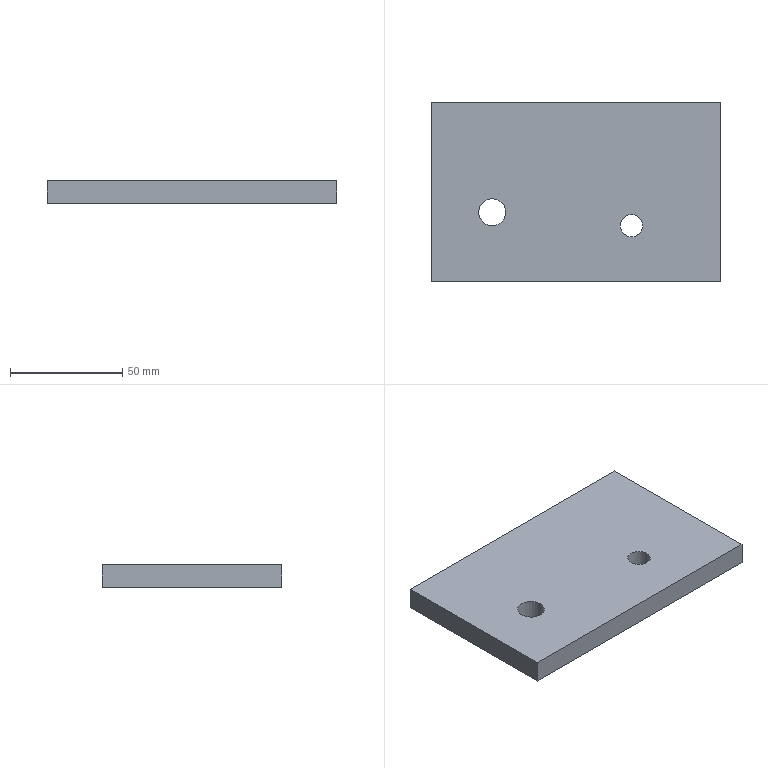Part | NX | features solid 2 | 1 solid | 8 faces | box 129 x 80 x 10 mm | volume 101284 mm3 | plane 6 | cylinder 2 | commonest cylinder face diameters 10 x1 12 x1
STEP:
#1=CARTESIAN_POINT('',(-391.,441.,-10.));
#2=VERTEX_POINT('',#1);
#3=CARTESIAN_POINT('',(-397.,441.,-10.));
#4=DIRECTION('',(0.,0.,1.));
#5=DIRECTION('',(1.,0.,0.));
#6=AXIS2_PLACEMENT_3D('',#3,#4,#5);
#7=CIRCLE('',#6,6.);
#8=EDGE_CURVE('',#2,#2,#7,.F.);
#9=ORIENTED_EDGE('',*,*,#8,.T.);
#10=EDGE_LOOP('',(#9));
#11=FACE_BOUND('',#10,.T.);
#12=CARTESIAN_POINT('',(-424.173,490.,-10.));
#13=VERTEX_POINT('',#12);
#14=CARTESIAN_POINT('',(-295.173,490.,-10.));
#15=VERTEX_POINT('',#14);
#16=CARTESIAN_POINT('',(-374.173,490.,-10.));
#17=DIRECTION('',(1.,0.,0.));
#18=VECTOR('',#17,1000.);
#19=LINE('',#16,#18);
#20=EDGE_CURVE('',#13,#15,#19,.T.);
#21=ORIENTED_EDGE('',*,*,#20,.F.);
#22=CARTESIAN_POINT('',(-424.173,410.,-10.));
#23=VERTEX_POINT('',#22);
#24=CARTESIAN_POINT('',(-424.173,460.,-10.));
#25=DIRECTION('',(0.,-1.,0.));
#26=VECTOR('',#25,1000.);
#27=LINE('',#24,#26);
#28=EDGE_CURVE('',#13,#23,#27,.T.);
#29=ORIENTED_EDGE('',*,*,#28,.T.);
#30=CARTESIAN_POINT('',(-295.173,410.,-10.));
#31=VERTEX_POINT('',#30);
#32=CARTESIAN_POINT('',(-374.173,410.,-10.));
#33=DIRECTION('',(-1.,0.,0.));
#34=VECTOR('',#33,1000.);
#35=LINE('',#32,#34);
#36=EDGE_CURVE('',#31,#23,#35,.T.);
#37=ORIENTED_EDGE('',*,*,#36,.F.);
#38=CARTESIAN_POINT('',(-295.173,410.,-10.));
#39=DIRECTION('',(0.,1.,0.));
#40=VECTOR('',#39,1000.);
#41=LINE('',#38,#40);
#42=EDGE_CURVE('',#31,#15,#41,.T.);
#43=ORIENTED_EDGE('',*,*,#42,.T.);
#44=EDGE_LOOP('',(#21,#29,#37,#43));
#45=FACE_BOUND('',#44,.T.);
#46=CARTESIAN_POINT('',(-330.,435.,-10.));
#47=VERTEX_POINT('',#46);
#48=CARTESIAN_POINT('',(-335.,435.,-10.));
#49=DIRECTION('',(0.,0.,1.));
#50=DIRECTION('',(1.,0.,0.));
#51=AXIS2_PLACEMENT_3D('',#48,#49,#50);
#52=CIRCLE('',#51,5.);
#53=EDGE_CURVE('',#47,#47,#52,.F.);
#54=ORIENTED_EDGE('',*,*,#53,.T.);
#55=EDGE_LOOP('',(#54));
#56=FACE_BOUND('',#55,.T.);
#57=CARTESIAN_POINT('',(-374.173,460.,-10.));
#58=DIRECTION('',(0.,0.,1.));
#59=DIRECTION('',(1.,0.,0.));
#60=AXIS2_PLACEMENT_3D('',#57,#58,#59);
#61=PLANE('',#60);
#62=ADVANCED_FACE('',(#11,#45,#56),#61,.T.);
#63=CARTESIAN_POINT('',(-424.173,490.,-20.));
#64=VERTEX_POINT('',#63);
#65=CARTESIAN_POINT('',(-424.173,410.,-20.));
#66=VERTEX_POINT('',#65);
#67=CARTESIAN_POINT('',(-424.173,460.,-20.));
#68=DIRECTION('',(0.,-1.,0.));
#69=VECTOR('',#68,1000.);
#70=LINE('',#67,#69);
#71=EDGE_CURVE('',#64,#66,#70,.T.);
#72=ORIENTED_EDGE('',*,*,#71,.F.);
#73=CARTESIAN_POINT('',(-295.173,490.,-20.));
#74=VERTEX_POINT('',#73);
#75=CARTESIAN_POINT('',(-374.173,490.,-20.));
#76=DIRECTION('',(1.,0.,0.));
#77=VECTOR('',#76,1000.);
#78=LINE('',#75,#77);
#79=EDGE_CURVE('',#64,#74,#78,.T.);
#80=ORIENTED_EDGE('',*,*,#79,.T.);
#81=CARTESIAN_POINT('',(-295.173,410.,-20.));
#82=VERTEX_POINT('',#81);
#83=CARTESIAN_POINT('',(-295.173,410.,-20.));
#84=DIRECTION('',(0.,1.,0.));
#85=VECTOR('',#84,1000.);
#86=LINE('',#83,#85);
#87=EDGE_CURVE('',#82,#74,#86,.T.);
#88=ORIENTED_EDGE('',*,*,#87,.F.);
#89=CARTESIAN_POINT('',(-374.173,410.,-20.));
#90=DIRECTION('',(-1.,0.,0.));
#91=VECTOR('',#90,1000.);
#92=LINE('',#89,#91);
#93=EDGE_CURVE('',#82,#66,#92,.T.);
#94=ORIENTED_EDGE('',*,*,#93,.T.);
#95=EDGE_LOOP('',(#72,#80,#88,#94));
#96=FACE_BOUND('',#95,.T.);
#97=CARTESIAN_POINT('',(-391.,441.,-20.));
#98=VERTEX_POINT('',#97);
#99=CARTESIAN_POINT('',(-397.,441.,-20.));
#100=DIRECTION('',(0.,0.,1.));
#101=DIRECTION('',(1.,0.,0.));
#102=AXIS2_PLACEMENT_3D('',#99,#100,#101);
#103=CIRCLE('',#102,6.);
#104=EDGE_CURVE('',#98,#98,#103,.F.);
#105=ORIENTED_EDGE('',*,*,#104,.F.);
#106=EDGE_LOOP('',(#105));
#107=FACE_BOUND('',#106,.T.);
#108=CARTESIAN_POINT('',(-330.,435.,-20.));
#109=VERTEX_POINT('',#108);
#110=CARTESIAN_POINT('',(-335.,435.,-20.));
#111=DIRECTION('',(0.,0.,-1.));
#112=DIRECTION('',(1.,0.,0.));
#113=AXIS2_PLACEMENT_3D('',#110,#111,#112);
#114=CIRCLE('',#113,5.);
#115=EDGE_CURVE('',#109,#109,#114,.T.);
#116=ORIENTED_EDGE('',*,*,#115,.F.);
#117=EDGE_LOOP('',(#116));
#118=FACE_BOUND('',#117,.T.);
#119=CARTESIAN_POINT('',(-374.173,460.,-20.));
#120=DIRECTION('',(0.,0.,1.));
#121=DIRECTION('',(1.,0.,0.));
#122=AXIS2_PLACEMENT_3D('',#119,#120,#121);
#123=PLANE('',#122);
#124=ADVANCED_FACE('',(#96,#107,#118),#123,.F.);
#125=ORIENTED_EDGE('',*,*,#87,.T.);
#126=CARTESIAN_POINT('',(-295.173,490.,-10.));
#127=DIRECTION('',(0.,0.,-1.));
#128=VECTOR('',#127,1000.);
#129=LINE('',#126,#128);
#130=EDGE_CURVE('',#15,#74,#129,.T.);
#131=ORIENTED_EDGE('',*,*,#130,.F.);
#132=ORIENTED_EDGE('',*,*,#42,.F.);
#133=CARTESIAN_POINT('',(-295.173,410.,-10.));
#134=DIRECTION('',(0.,0.,-1.));
#135=VECTOR('',#134,1000.);
#136=LINE('',#133,#135);
#137=EDGE_CURVE('',#31,#82,#136,.T.);
#138=ORIENTED_EDGE('',*,*,#137,.T.);
#139=EDGE_LOOP('',(#125,#131,#132,#138));
#140=FACE_BOUND('',#139,.T.);
#141=CARTESIAN_POINT('',(-295.173,410.,-10.));
#142=DIRECTION('',(-1.,0.,0.));
#143=DIRECTION('',(0.,-1.,0.));
#144=AXIS2_PLACEMENT_3D('',#141,#142,#143);
#145=PLANE('',#144);
#146=ADVANCED_FACE('',(#140),#145,.F.);
#147=ORIENTED_EDGE('',*,*,#71,.T.);
#148=CARTESIAN_POINT('',(-424.173,410.,-10.));
#149=DIRECTION('',(0.,0.,-1.));
#150=VECTOR('',#149,1000.);
#151=LINE('',#148,#150);
#152=EDGE_CURVE('',#23,#66,#151,.T.);
#153=ORIENTED_EDGE('',*,*,#152,.F.);
#154=ORIENTED_EDGE('',*,*,#28,.F.);
#155=CARTESIAN_POINT('',(-424.173,490.,-10.));
#156=DIRECTION('',(0.,0.,-1.));
#157=VECTOR('',#156,1000.);
#158=LINE('',#155,#157);
#159=EDGE_CURVE('',#13,#64,#158,.T.);
#160=ORIENTED_EDGE('',*,*,#159,.T.);
#161=EDGE_LOOP('',(#147,#153,#154,#160));
#162=FACE_BOUND('',#161,.T.);
#163=CARTESIAN_POINT('',(-424.173,460.,-10.));
#164=DIRECTION('',(1.,0.,0.));
#165=DIRECTION('',(0.,1.,0.));
#166=AXIS2_PLACEMENT_3D('',#163,#164,#165);
#167=PLANE('',#166);
#168=ADVANCED_FACE('',(#162),#167,.F.);
#169=ORIENTED_EDGE('',*,*,#137,.F.);
#170=ORIENTED_EDGE('',*,*,#36,.T.);
#171=ORIENTED_EDGE('',*,*,#152,.T.);
#172=ORIENTED_EDGE('',*,*,#93,.F.);
#173=EDGE_LOOP('',(#169,#170,#171,#172));
#174=FACE_BOUND('',#173,.T.);
#175=CARTESIAN_POINT('',(-374.173,410.,-10.));
#176=DIRECTION('',(0.,1.,0.));
#177=DIRECTION('',(-1.,0.,0.));
#178=AXIS2_PLACEMENT_3D('',#175,#176,#177);
#179=PLANE('',#178);
#180=ADVANCED_FACE('',(#174),#179,.F.);
#181=ORIENTED_EDGE('',*,*,#8,.F.);
#182=EDGE_LOOP('',(#181));
#183=FACE_BOUND('',#182,.T.);
#184=ORIENTED_EDGE('',*,*,#104,.T.);
#185=EDGE_LOOP('',(#184));
#186=FACE_BOUND('',#185,.T.);
#187=CARTESIAN_POINT('',(-397.,441.,55.));
#188=DIRECTION('',(0.,0.,-1.));
#189=DIRECTION('',(1.,0.,0.));
#190=AXIS2_PLACEMENT_3D('',#187,#188,#189);
#191=CYLINDRICAL_SURFACE('',#190,6.);
#192=ADVANCED_FACE('',(#183,#186),#191,.F.);
#193=ORIENTED_EDGE('',*,*,#159,.F.);
#194=ORIENTED_EDGE('',*,*,#20,.T.);
#195=ORIENTED_EDGE('',*,*,#130,.T.);
#196=ORIENTED_EDGE('',*,*,#79,.F.);
#197=EDGE_LOOP('',(#193,#194,#195,#196));
#198=FACE_BOUND('',#197,.T.);
#199=CARTESIAN_POINT('',(-295.173,490.,-10.));
#200=DIRECTION('',(0.,-1.,0.));
#201=DIRECTION('',(1.,0.,0.));
#202=AXIS2_PLACEMENT_3D('',#199,#200,#201);
#203=PLANE('',#202);
#204=ADVANCED_FACE('',(#198),#203,.F.);
#205=ORIENTED_EDGE('',*,*,#53,.F.);
#206=EDGE_LOOP('',(#205));
#207=FACE_BOUND('',#206,.T.);
#208=ORIENTED_EDGE('',*,*,#115,.T.);
#209=EDGE_LOOP('',(#208));
#210=FACE_BOUND('',#209,.T.);
#211=CARTESIAN_POINT('',(-335.,435.,-20.));
#212=DIRECTION('',(0.,0.,1.));
#213=DIRECTION('',(1.,0.,0.));
#214=AXIS2_PLACEMENT_3D('',#211,#212,#213);
#215=CYLINDRICAL_SURFACE('',#214,5.);
#216=ADVANCED_FACE('',(#207,#210),#215,.F.);
#217=CLOSED_SHELL('',(#62,#124,#146,#168,#180,#192,#204,#216));
#218=MANIFOLD_SOLID_BREP('',#217);
#219=(LENGTH_UNIT()NAMED_UNIT(*)SI_UNIT(.MILLI.,.METRE.));
#220=UNCERTAINTY_MEASURE_WITH_UNIT(LENGTH_MEASURE(0.00001),#219,'','');
#221=(NAMED_UNIT(*)PLANE_ANGLE_UNIT()SI_UNIT($,.RADIAN.));
#222=(NAMED_UNIT(*)SI_UNIT($,.STERADIAN.)SOLID_ANGLE_UNIT());
#223=(GEOMETRIC_REPRESENTATION_CONTEXT(3)GLOBAL_UNCERTAINTY_ASSIGNED_CONTEXT((#220))GLOBAL_UNIT_ASSIGNED_CONTEXT((#219,#221,#222))REPRESENTATION_CONTEXT('',''));
#224=ADVANCED_BREP_SHAPE_REPRESENTATION('',(#218),#223);